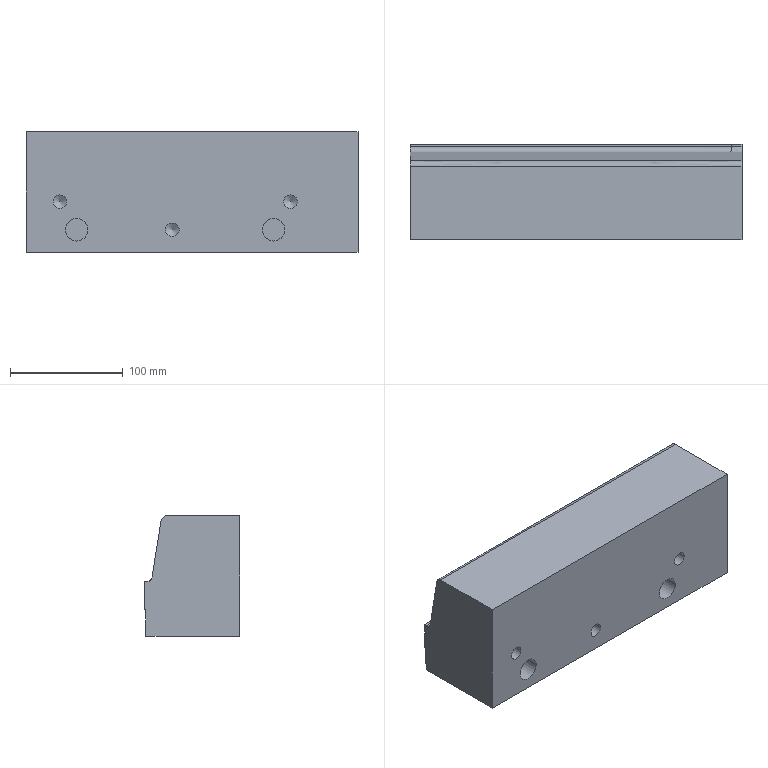Part | NX | features solid 2 | 1 solid | 24 faces | box 295 x 84.705 x 107.133 mm | volume 2449051 mm3 | plane 9 | cylinder 6 | spline 6 | cone 3 | commonest cylinder face diameters 12 x3 20 x2 10 x1
STEP:
#1=CARTESIAN_POINT('',(370.,-160.,-50.));
#2=VERTEX_POINT('',#1);
#3=CARTESIAN_POINT('',(370.,-76.709,-50.));
#4=VERTEX_POINT('',#3);
#5=CARTESIAN_POINT('',(370.,-159.,-50.));
#6=DIRECTION('',(0.,1.,0.));
#7=VECTOR('',#6,1000.);
#8=LINE('',#5,#7);
#9=EDGE_CURVE('',#2,#4,#8,.T.);
#10=ORIENTED_EDGE('',*,*,#9,.T.);
#11=CARTESIAN_POINT('',(665.,-76.708,-50.));
#12=VERTEX_POINT('',#11);
#13=CARTESIAN_POINT('',(370.,-76.709,-50.));
#14=CARTESIAN_POINT('',(468.333,-76.709,-50.));
#15=CARTESIAN_POINT('',(566.667,-76.708,-50.));
#16=CARTESIAN_POINT('',(665.,-76.708,-50.));
#17=B_SPLINE_CURVE_WITH_KNOTS('',3,(#13,#14,#15,#16),.UNSPECIFIED.,.F.,.F.,(4,4),(0.146,0.441),.UNSPECIFIED.);
#18=EDGE_CURVE('',#4,#12,#17,.T.);
#19=ORIENTED_EDGE('',*,*,#18,.T.);
#20=CARTESIAN_POINT('',(665.,-160.,-50.));
#21=VERTEX_POINT('',#20);
#22=CARTESIAN_POINT('',(665.,-74.471,-50.));
#23=DIRECTION('',(0.,1.,0.));
#24=VECTOR('',#23,1000.);
#25=LINE('',#22,#24);
#26=EDGE_CURVE('',#21,#12,#25,.T.);
#27=ORIENTED_EDGE('',*,*,#26,.F.);
#28=CARTESIAN_POINT('',(-571.479,-160.,-50.));
#29=DIRECTION('',(1.,0.,0.));
#30=VECTOR('',#29,1000.);
#31=LINE('',#28,#30);
#32=EDGE_CURVE('',#2,#21,#31,.T.);
#33=ORIENTED_EDGE('',*,*,#32,.F.);
#34=EDGE_LOOP('',(#10,#19,#27,#33));
#35=FACE_BOUND('',#34,.T.);
#36=CARTESIAN_POINT('',(-571.479,-74.471,-50.));
#37=DIRECTION('',(0.,0.,-1.));
#38=DIRECTION('',(-1.,0.,0.));
#39=AXIS2_PLACEMENT_3D('',#36,#37,#38);
#40=PLANE('',#39);
#41=ADVANCED_FACE('',(#35),#40,.T.);
#42=CARTESIAN_POINT('',(415.,-160.,-20.));
#43=VERTEX_POINT('',#42);
#44=CARTESIAN_POINT('',(415.,-160.,-30.));
#45=DIRECTION('',(0.,1.,0.));
#46=DIRECTION('',(0.,0.,1.));
#47=AXIS2_PLACEMENT_3D('',#44,#45,#46);
#48=CIRCLE('',#47,10.);
#49=EDGE_CURVE('',#43,#43,#48,.T.);
#50=ORIENTED_EDGE('',*,*,#49,.T.);
#51=EDGE_LOOP('',(#50));
#52=FACE_BOUND('',#51,.T.);
#53=CARTESIAN_POINT('',(590.,-160.,-20.));
#54=VERTEX_POINT('',#53);
#55=CARTESIAN_POINT('',(590.,-160.,-30.));
#56=DIRECTION('',(0.,1.,0.));
#57=DIRECTION('',(0.,0.,1.));
#58=AXIS2_PLACEMENT_3D('',#55,#56,#57);
#59=CIRCLE('',#58,10.);
#60=EDGE_CURVE('',#54,#54,#59,.T.);
#61=ORIENTED_EDGE('',*,*,#60,.T.);
#62=EDGE_LOOP('',(#61));
#63=FACE_BOUND('',#62,.T.);
#64=CARTESIAN_POINT('',(400.,-160.,1.));
#65=VERTEX_POINT('',#64);
#66=CARTESIAN_POINT('',(400.,-160.,-5.));
#67=DIRECTION('',(0.,1.,0.));
#68=DIRECTION('',(0.,0.,1.));
#69=AXIS2_PLACEMENT_3D('',#66,#67,#68);
#70=CIRCLE('',#69,6.);
#71=EDGE_CURVE('',#65,#65,#70,.T.);
#72=ORIENTED_EDGE('',*,*,#71,.T.);
#73=EDGE_LOOP('',(#72));
#74=FACE_BOUND('',#73,.T.);
#75=CARTESIAN_POINT('',(500.,-160.,-24.));
#76=VERTEX_POINT('',#75);
#77=CARTESIAN_POINT('',(500.,-160.,-30.));
#78=DIRECTION('',(0.,1.,0.));
#79=DIRECTION('',(0.,0.,1.));
#80=AXIS2_PLACEMENT_3D('',#77,#78,#79);
#81=CIRCLE('',#80,6.);
#82=EDGE_CURVE('',#76,#76,#81,.T.);
#83=ORIENTED_EDGE('',*,*,#82,.T.);
#84=EDGE_LOOP('',(#83));
#85=FACE_BOUND('',#84,.T.);
#86=CARTESIAN_POINT('',(605.,-160.,1.));
#87=VERTEX_POINT('',#86);
#88=CARTESIAN_POINT('',(605.,-160.,-5.));
#89=DIRECTION('',(0.,1.,0.));
#90=DIRECTION('',(0.,0.,1.));
#91=AXIS2_PLACEMENT_3D('',#88,#89,#90);
#92=CIRCLE('',#91,6.);
#93=EDGE_CURVE('',#87,#87,#92,.T.);
#94=ORIENTED_EDGE('',*,*,#93,.T.);
#95=EDGE_LOOP('',(#94));
#96=FACE_BOUND('',#95,.T.);
#97=ORIENTED_EDGE('',*,*,#32,.T.);
#98=CARTESIAN_POINT('',(665.,-160.,57.133));
#99=VERTEX_POINT('',#98);
#100=CARTESIAN_POINT('',(665.,-160.,200.));
#101=DIRECTION('',(0.,0.,-1.));
#102=VECTOR('',#101,1000.);
#103=LINE('',#100,#102);
#104=EDGE_CURVE('',#99,#21,#103,.T.);
#105=ORIENTED_EDGE('',*,*,#104,.F.);
#106=CARTESIAN_POINT('',(370.,-160.,57.133));
#107=VERTEX_POINT('',#106);
#108=CARTESIAN_POINT('',(-705.,-160.,57.133));
#109=DIRECTION('',(1.,0.,0.));
#110=VECTOR('',#109,1000.);
#111=LINE('',#108,#110);
#112=EDGE_CURVE('',#107,#99,#111,.T.);
#113=ORIENTED_EDGE('',*,*,#112,.F.);
#114=CARTESIAN_POINT('',(370.,-160.,200.));
#115=DIRECTION('',(0.,0.,1.));
#116=VECTOR('',#115,1000.);
#117=LINE('',#114,#116);
#118=EDGE_CURVE('',#2,#107,#117,.T.);
#119=ORIENTED_EDGE('',*,*,#118,.F.);
#120=EDGE_LOOP('',(#97,#105,#113,#119));
#121=FACE_BOUND('',#120,.T.);
#122=CARTESIAN_POINT('',(-705.,-160.,200.));
#123=DIRECTION('',(0.,1.,0.));
#124=DIRECTION('',(0.,0.,1.));
#125=AXIS2_PLACEMENT_3D('',#122,#123,#124);
#126=PLANE('',#125);
#127=ADVANCED_FACE('',(#52,#63,#74,#85,#96,#121),#126,.F.);
#128=CARTESIAN_POINT('',(370.,-77.294,-1.492));
#129=VERTEX_POINT('',#128);
#130=CARTESIAN_POINT('',(370.,-75.295,-1.509));
#131=VERTEX_POINT('',#130);
#132=CARTESIAN_POINT('',(370.,47.797,-2.56));
#133=DIRECTION('',(0.,1.,-0.008536));
#134=VECTOR('',#133,1000.);
#135=LINE('',#132,#134);
#136=EDGE_CURVE('',#129,#131,#135,.T.);
#137=ORIENTED_EDGE('',*,*,#136,.F.);
#138=CARTESIAN_POINT('',(655.556,-77.294,-1.492));
#139=VERTEX_POINT('',#138);
#140=CARTESIAN_POINT('',(655.556,-77.294,-1.492));
#141=CARTESIAN_POINT('',(560.371,-77.294,-1.492));
#142=CARTESIAN_POINT('',(465.185,-77.294,-1.492));
#143=CARTESIAN_POINT('',(370.,-77.294,-1.492));
#144=B_SPLINE_CURVE_WITH_KNOTS('',3,(#140,#141,#142,#143),.UNSPECIFIED.,.F.,.F.,(4,4),(0.,0.3388),.UNSPECIFIED.);
#145=EDGE_CURVE('',#139,#129,#144,.T.);
#146=ORIENTED_EDGE('',*,*,#145,.F.);
#147=CARTESIAN_POINT('',(655.585,-75.295,-1.509));
#148=VERTEX_POINT('',#147);
#149=CARTESIAN_POINT('',(655.585,-75.295,-1.509));
#150=CARTESIAN_POINT('',(655.576,-75.961,-1.503));
#151=CARTESIAN_POINT('',(655.566,-76.628,-1.498));
#152=CARTESIAN_POINT('',(655.556,-77.294,-1.492));
#153=B_SPLINE_CURVE_WITH_KNOTS('',3,(#149,#150,#151,#152),.UNSPECIFIED.,.F.,.F.,(4,4),(0.8984,1.),.UNSPECIFIED.);
#154=EDGE_CURVE('',#148,#139,#153,.T.);
#155=ORIENTED_EDGE('',*,*,#154,.F.);
#156=CARTESIAN_POINT('',(370.,-75.295,-1.509));
#157=CARTESIAN_POINT('',(465.195,-75.295,-1.509));
#158=CARTESIAN_POINT('',(560.39,-75.295,-1.509));
#159=CARTESIAN_POINT('',(655.585,-75.295,-1.509));
#160=B_SPLINE_CURVE_WITH_KNOTS('',3,(#156,#157,#158,#159),.UNSPECIFIED.,.F.,.F.,(4,4),(0.7675,1.053),.UNSPECIFIED.);
#161=EDGE_CURVE('',#131,#148,#160,.T.);
#162=ORIENTED_EDGE('',*,*,#161,.F.);
#163=EDGE_LOOP('',(#137,#146,#155,#162));
#164=FACE_BOUND('',#163,.T.);
#165=CARTESIAN_POINT('',(35.495,47.797,-2.56));
#166=DIRECTION('',(0.,-0.008536,-1.));
#167=DIRECTION('',(0.,-1.,0.008536));
#168=AXIS2_PLACEMENT_3D('',#165,#166,#167);
#169=PLANE('',#168);
#170=ADVANCED_FACE('',(#164),#169,.F.);
#171=CARTESIAN_POINT('',(370.,-82.189,2.72));
#172=VERTEX_POINT('',#171);
#173=CARTESIAN_POINT('',(370.,-77.252,3.508));
#174=DIRECTION('',(-1.,0.,0.));
#175=DIRECTION('',(0.,0.,1.));
#176=AXIS2_PLACEMENT_3D('',#173,#174,#175);
#177=CIRCLE('',#176,5.);
#178=EDGE_CURVE('',#172,#129,#177,.F.);
#179=ORIENTED_EDGE('',*,*,#178,.F.);
#180=CARTESIAN_POINT('',(655.125,-82.189,2.72));
#181=VERTEX_POINT('',#180);
#182=CARTESIAN_POINT('',(370.,-82.189,2.72));
#183=CARTESIAN_POINT('',(465.042,-82.189,2.72));
#184=CARTESIAN_POINT('',(560.083,-82.189,2.72));
#185=CARTESIAN_POINT('',(655.125,-82.189,2.72));
#186=B_SPLINE_CURVE_WITH_KNOTS('',3,(#182,#183,#184,#185),.UNSPECIFIED.,.F.,.F.,(4,4),(0.6615,1.),.UNSPECIFIED.);
#187=EDGE_CURVE('',#172,#181,#186,.T.);
#188=ORIENTED_EDGE('',*,*,#187,.T.);
#189=CARTESIAN_POINT('',(655.125,-82.189,2.72));
#190=CARTESIAN_POINT('',(655.257,-81.952,1.234));
#191=CARTESIAN_POINT('',(655.46,-80.192,-1.055));
#192=CARTESIAN_POINT('',(655.544,-78.13,-1.485));
#193=CARTESIAN_POINT('',(655.556,-77.294,-1.492));
#194=B_SPLINE_CURVE_WITH_KNOTS('',3,(#189,#190,#191,#192,#193),.UNSPECIFIED.,.F.,.F.,(4,1,4),(0.,0.5,1.),.UNSPECIFIED.);
#195=EDGE_CURVE('',#181,#139,#194,.T.);
#196=ORIENTED_EDGE('',*,*,#195,.T.);
#197=ORIENTED_EDGE('',*,*,#145,.T.);
#198=EDGE_LOOP('',(#179,#188,#196,#197));
#199=FACE_BOUND('',#198,.T.);
#200=CARTESIAN_POINT('',(6000655.556,-77.252,3.508));
#201=DIRECTION('',(-1.,0.,0.));
#202=DIRECTION('',(0.,-0.1575,0.9875));
#203=AXIS2_PLACEMENT_3D('',#200,#201,#202);
#204=CYLINDRICAL_SURFACE('',#203,5.);
#205=ADVANCED_FACE('',(#199),#204,.F.);
#206=CARTESIAN_POINT('',(370.,-90.197,52.92));
#207=VERTEX_POINT('',#206);
#208=CARTESIAN_POINT('',(665.,-90.197,52.92));
#209=VERTEX_POINT('',#208);
#210=CARTESIAN_POINT('',(370.,-90.197,52.92));
#211=CARTESIAN_POINT('',(468.333,-90.197,52.92));
#212=CARTESIAN_POINT('',(566.667,-90.197,52.92));
#213=CARTESIAN_POINT('',(665.,-90.197,52.92));
#214=B_SPLINE_CURVE_WITH_KNOTS('',3,(#210,#211,#212,#213),.UNSPECIFIED.,.F.,.F.,(4,4),(0.5681,0.8631),.UNSPECIFIED.);
#215=EDGE_CURVE('',#207,#209,#214,.T.);
#216=ORIENTED_EDGE('',*,*,#215,.F.);
#217=CARTESIAN_POINT('',(370.,-95.134,57.133));
#218=VERTEX_POINT('',#217);
#219=CARTESIAN_POINT('',(370.,-95.134,52.133));
#220=DIRECTION('',(-1.,0.,0.));
#221=DIRECTION('',(0.,0.,1.));
#222=AXIS2_PLACEMENT_3D('',#219,#220,#221);
#223=CIRCLE('',#222,5.);
#224=EDGE_CURVE('',#207,#218,#223,.F.);
#225=ORIENTED_EDGE('',*,*,#224,.T.);
#226=CARTESIAN_POINT('',(665.,-95.134,57.133));
#227=VERTEX_POINT('',#226);
#228=CARTESIAN_POINT('',(665.,-95.134,57.133));
#229=CARTESIAN_POINT('',(566.667,-95.134,57.133));
#230=CARTESIAN_POINT('',(468.333,-95.134,57.133));
#231=CARTESIAN_POINT('',(370.,-95.134,57.133));
#232=B_SPLINE_CURVE_WITH_KNOTS('',3,(#228,#229,#230,#231),.UNSPECIFIED.,.F.,.F.,(4,4),(0.07861,0.3736),.UNSPECIFIED.);
#233=EDGE_CURVE('',#227,#218,#232,.T.);
#234=ORIENTED_EDGE('',*,*,#233,.F.);
#235=CARTESIAN_POINT('',(665.,-95.134,52.133));
#236=DIRECTION('',(-1.,0.,0.));
#237=DIRECTION('',(0.,0.,1.));
#238=AXIS2_PLACEMENT_3D('',#235,#236,#237);
#239=CIRCLE('',#238,5.);
#240=EDGE_CURVE('',#227,#209,#239,.T.);
#241=ORIENTED_EDGE('',*,*,#240,.T.);
#242=EDGE_LOOP('',(#216,#225,#234,#241));
#243=FACE_BOUND('',#242,.T.);
#244=CARTESIAN_POINT('',(665.,-90.197,52.92));
#245=CARTESIAN_POINT('',(665.,-90.869,57.133));
#246=CARTESIAN_POINT('',(665.,-95.134,57.133));
#247=CARTESIAN_POINT('',(566.667,-90.197,52.92));
#248=CARTESIAN_POINT('',(566.667,-90.869,57.133));
#249=CARTESIAN_POINT('',(566.667,-95.134,57.133));
#250=CARTESIAN_POINT('',(468.333,-90.197,52.92));
#251=CARTESIAN_POINT('',(468.333,-90.869,57.133));
#252=CARTESIAN_POINT('',(468.333,-95.134,57.133));
#253=CARTESIAN_POINT('',(370.,-90.197,52.92));
#254=CARTESIAN_POINT('',(370.,-90.869,57.133));
#255=CARTESIAN_POINT('',(370.,-95.134,57.133));
#256=(BOUNDED_SURFACE()B_SPLINE_SURFACE(3,2,((#244,#245,#246),(#247,#248,#249),(#250,#251,#252),(#253,#254,#255)),.UNSPECIFIED.,.F.,.F.,.F.)B_SPLINE_SURFACE_WITH_KNOTS((4,4),(3,3),(0.1943,0.4893),(0.,1.),.PIECEWISE_BEZIER_KNOTS.)GEOMETRIC_REPRESENTATION_ITEM()RATIONAL_B_SPLINE_SURFACE(((1.,0.7608,1.),(1.,0.7608,1.),(1.,0.7608,1.),(1.,0.7608,1.)))REPRESENTATION_ITEM('')SURFACE());
#257=ADVANCED_FACE('',(#243),#256,.T.);
#258=CARTESIAN_POINT('',(370.,-86.499,29.736));
#259=DIRECTION('',(0.,0.1575,-0.9875));
#260=VECTOR('',#259,1000.);
#261=LINE('',#258,#260);
#262=EDGE_CURVE('',#207,#172,#261,.T.);
#263=ORIENTED_EDGE('',*,*,#262,.F.);
#264=ORIENTED_EDGE('',*,*,#215,.T.);
#265=CARTESIAN_POINT('',(665.,-82.189,2.72));
#266=VERTEX_POINT('',#265);
#267=CARTESIAN_POINT('',(665.,-90.197,52.92));
#268=CARTESIAN_POINT('',(665.,-87.528,36.187));
#269=CARTESIAN_POINT('',(665.,-84.858,19.454));
#270=CARTESIAN_POINT('',(665.,-82.189,2.72));
#271=B_SPLINE_CURVE_WITH_KNOTS('',3,(#267,#268,#269,#270),.UNSPECIFIED.,.F.,.F.,(4,4),(0.1423,0.1932),.UNSPECIFIED.);
#272=EDGE_CURVE('',#266,#209,#271,.F.);
#273=ORIENTED_EDGE('',*,*,#272,.F.);
#274=CARTESIAN_POINT('',(655.125,-82.189,2.72));
#275=CARTESIAN_POINT('',(658.417,-82.189,2.72));
#276=CARTESIAN_POINT('',(661.708,-82.189,2.72));
#277=CARTESIAN_POINT('',(665.,-82.189,2.72));
#278=B_SPLINE_CURVE_WITH_KNOTS('',3,(#274,#275,#276,#277),.UNSPECIFIED.,.F.,.F.,(4,4),(0.9354,0.9453),.UNSPECIFIED.);
#279=EDGE_CURVE('',#181,#266,#278,.T.);
#280=ORIENTED_EDGE('',*,*,#279,.F.);
#281=ORIENTED_EDGE('',*,*,#187,.F.);
#282=EDGE_LOOP('',(#263,#264,#273,#280,#281));
#283=FACE_BOUND('',#282,.T.);
#284=CARTESIAN_POINT('',(808.196,-81.695,-0.3814));
#285=CARTESIAN_POINT('',(-199.284,-81.695,-0.3814));
#286=CARTESIAN_POINT('',(808.196,-91.303,59.853));
#287=CARTESIAN_POINT('',(-199.284,-91.303,59.853));
#288=B_SPLINE_SURFACE_WITH_KNOTS('',1,1,((#284,#285),(#286,#287)),.PLANE_SURF.,.F.,.F.,.F.,(2,2),(2,2),(-0.06964,1.283),(-0.1722,1.),.UNSPECIFIED.);
#289=ADVANCED_FACE('',(#283),#288,.F.);
#290=CARTESIAN_POINT('',(665.,-77.294,-1.492));
#291=VERTEX_POINT('',#290);
#292=CARTESIAN_POINT('',(665.,-77.252,3.508));
#293=DIRECTION('',(-1.,0.,0.));
#294=DIRECTION('',(0.,0.,1.));
#295=AXIS2_PLACEMENT_3D('',#292,#293,#294);
#296=CIRCLE('',#295,5.);
#297=EDGE_CURVE('',#291,#266,#296,.T.);
#298=ORIENTED_EDGE('',*,*,#297,.F.);
#299=CARTESIAN_POINT('',(655.556,-77.294,-1.492));
#300=CARTESIAN_POINT('',(658.704,-77.294,-1.492));
#301=CARTESIAN_POINT('',(661.852,-77.294,-1.492));
#302=CARTESIAN_POINT('',(665.,-77.294,-1.492));
#303=B_SPLINE_CURVE_WITH_KNOTS('',3,(#299,#300,#301,#302),.UNSPECIFIED.,.F.,.F.,(4,4),(0.,0.1078),.UNSPECIFIED.);
#304=EDGE_CURVE('',#139,#291,#303,.T.);
#305=ORIENTED_EDGE('',*,*,#304,.F.);
#306=ORIENTED_EDGE('',*,*,#195,.F.);
#307=ORIENTED_EDGE('',*,*,#279,.T.);
#308=EDGE_LOOP('',(#298,#305,#306,#307));
#309=FACE_BOUND('',#308,.T.);
#310=CARTESIAN_POINT('',(665.,-82.189,2.72));
#311=CARTESIAN_POINT('',(665.,-81.523,-1.456));
#312=CARTESIAN_POINT('',(665.,-77.294,-1.492));
#313=CARTESIAN_POINT('',(661.689,-82.189,2.72));
#314=CARTESIAN_POINT('',(661.689,-81.523,-1.456));
#315=CARTESIAN_POINT('',(661.689,-77.294,-1.492));
#316=CARTESIAN_POINT('',(658.377,-82.189,2.72));
#317=CARTESIAN_POINT('',(658.377,-81.523,-1.456));
#318=CARTESIAN_POINT('',(658.377,-77.294,-1.492));
#319=CARTESIAN_POINT('',(655.066,-82.189,2.72));
#320=CARTESIAN_POINT('',(655.066,-81.523,-1.456));
#321=CARTESIAN_POINT('',(655.066,-77.294,-1.492));
#322=(BOUNDED_SURFACE()B_SPLINE_SURFACE(3,2,((#310,#311,#312),(#313,#314,#315),(#316,#317,#318),(#319,#320,#321)),.UNSPECIFIED.,.F.,.F.,.F.)B_SPLINE_SURFACE_WITH_KNOTS((4,4),(3,3),(0.4081,0.418),(0.,1.),.PIECEWISE_BEZIER_KNOTS.)GEOMETRIC_REPRESENTATION_ITEM()RATIONAL_B_SPLINE_SURFACE(((1.,0.7635,1.),(1.,0.7635,1.),(1.,0.7635,1.),(1.,0.7635,1.)))REPRESENTATION_ITEM('')SURFACE());
#323=ADVANCED_FACE('',(#309),#322,.F.);
#324=CARTESIAN_POINT('',(665.,-75.295,-1.509));
#325=VERTEX_POINT('',#324);
#326=CARTESIAN_POINT('',(655.585,-75.295,-1.509));
#327=CARTESIAN_POINT('',(658.724,-75.295,-1.509));
#328=CARTESIAN_POINT('',(661.862,-75.295,-1.509));
#329=CARTESIAN_POINT('',(665.,-75.295,-1.509));
#330=B_SPLINE_CURVE_WITH_KNOTS('',3,(#326,#327,#328,#329),.UNSPECIFIED.,.F.,.F.,(4,4),(0.000855,0.01027),.UNSPECIFIED.);
#331=EDGE_CURVE('',#148,#325,#330,.T.);
#332=ORIENTED_EDGE('',*,*,#331,.F.);
#333=ORIENTED_EDGE('',*,*,#154,.T.);
#334=ORIENTED_EDGE('',*,*,#304,.T.);
#335=CARTESIAN_POINT('',(665.,-75.295,-1.509));
#336=CARTESIAN_POINT('',(665.,-75.961,-1.503));
#337=CARTESIAN_POINT('',(665.,-76.628,-1.498));
#338=CARTESIAN_POINT('',(665.,-77.294,-1.492));
#339=B_SPLINE_CURVE_WITH_KNOTS('',3,(#335,#336,#337,#338),.UNSPECIFIED.,.F.,.F.,(4,4),(0.01519,0.01719),.UNSPECIFIED.);
#340=EDGE_CURVE('',#325,#291,#339,.T.);
#341=ORIENTED_EDGE('',*,*,#340,.F.);
#342=EDGE_LOOP('',(#332,#333,#334,#341));
#343=FACE_BOUND('',#342,.T.);
#344=CARTESIAN_POINT('',(665.,-75.295,-1.509));
#345=CARTESIAN_POINT('',(655.5,-75.295,-1.509));
#346=CARTESIAN_POINT('',(665.,-77.294,-1.492));
#347=CARTESIAN_POINT('',(655.5,-77.294,-1.492));
#348=B_SPLINE_SURFACE_WITH_KNOTS('',1,1,((#344,#345),(#346,#347)),.PLANE_SURF.,.F.,.F.,.F.,(2,2),(2,2),(0.6913,0.7357),(0.06336,0.0699),.PIECEWISE_BEZIER_KNOTS.);
#349=ADVANCED_FACE('',(#343),#348,.F.);
#350=CARTESIAN_POINT('',(370.,-75.295,-26.51));
#351=VERTEX_POINT('',#350);
#352=CARTESIAN_POINT('',(370.,-75.295,-14.009));
#353=DIRECTION('',(0.,0.,-1.));
#354=VECTOR('',#353,1000.);
#355=LINE('',#352,#354);
#356=EDGE_CURVE('',#131,#351,#355,.T.);
#357=ORIENTED_EDGE('',*,*,#356,.F.);
#358=ORIENTED_EDGE('',*,*,#161,.T.);
#359=ORIENTED_EDGE('',*,*,#331,.T.);
#360=CARTESIAN_POINT('',(665.,-75.295,-26.51));
#361=VERTEX_POINT('',#360);
#362=CARTESIAN_POINT('',(665.,-75.295,-14.009));
#363=DIRECTION('',(0.,0.,-1.));
#364=VECTOR('',#363,1000.);
#365=LINE('',#362,#364);
#366=EDGE_CURVE('',#325,#361,#365,.T.);
#367=ORIENTED_EDGE('',*,*,#366,.T.);
#368=CARTESIAN_POINT('',(665.,-75.295,-26.51));
#369=CARTESIAN_POINT('',(566.667,-75.295,-26.51));
#370=CARTESIAN_POINT('',(468.333,-75.295,-26.51));
#371=CARTESIAN_POINT('',(370.,-75.295,-26.51));
#372=B_SPLINE_CURVE_WITH_KNOTS('',3,(#368,#369,#370,#371),.UNSPECIFIED.,.F.,.F.,(4,4),(-0.005,0.29),.UNSPECIFIED.);
#373=EDGE_CURVE('',#361,#351,#372,.T.);
#374=ORIENTED_EDGE('',*,*,#373,.T.);
#375=EDGE_LOOP('',(#357,#358,#359,#367,#374));
#376=FACE_BOUND('',#375,.T.);
#377=CARTESIAN_POINT('',(665.,-75.295,-1.509));
#378=CARTESIAN_POINT('',(665.,-75.295,-26.51));
#379=CARTESIAN_POINT('',(663.333,-75.295,-1.509));
#380=CARTESIAN_POINT('',(663.333,-75.295,-26.51));
#381=CARTESIAN_POINT('',(661.667,-75.295,-1.509));
#382=CARTESIAN_POINT('',(661.667,-75.295,-26.51));
#383=CARTESIAN_POINT('',(660.,-75.295,-1.509));
#384=CARTESIAN_POINT('',(660.,-75.295,-26.51));
#385=CARTESIAN_POINT('',(563.333,-75.295,-1.509));
#386=CARTESIAN_POINT('',(563.333,-75.295,-26.51));
#387=CARTESIAN_POINT('',(466.667,-75.295,-1.509));
#388=CARTESIAN_POINT('',(466.667,-75.295,-26.51));
#389=CARTESIAN_POINT('',(370.,-75.295,-1.509));
#390=CARTESIAN_POINT('',(370.,-75.295,-26.51));
#391=B_SPLINE_SURFACE_WITH_KNOTS('',3,1,((#377,#378),(#379,#380),(#381,#382),(#383,#384),(#385,#386),(#387,#388),(#389,#390)),.SURF_OF_LINEAR_EXTRUSION.,.F.,.F.,.F.,(4,3,4),(2,2),(-0.003661,0.,0.2124),(0.,1.),.PIECEWISE_BEZIER_KNOTS.);
#392=ADVANCED_FACE('',(#376),#391,.F.);
#393=ORIENTED_EDGE('',*,*,#18,.F.);
#394=CARTESIAN_POINT('',(370.,-76.508,-26.5));
#395=VERTEX_POINT('',#394);
#396=CARTESIAN_POINT('',(370.,-76.709,-50.));
#397=DIRECTION('',(0.,-0.008536,-1.));
#398=VECTOR('',#397,1000.);
#399=LINE('',#396,#398);
#400=EDGE_CURVE('',#4,#395,#399,.F.);
#401=ORIENTED_EDGE('',*,*,#400,.T.);
#402=CARTESIAN_POINT('',(665.,-76.508,-26.5));
#403=VERTEX_POINT('',#402);
#404=CARTESIAN_POINT('',(665.,-76.508,-26.5));
#405=CARTESIAN_POINT('',(566.667,-76.508,-26.5));
#406=CARTESIAN_POINT('',(468.333,-76.508,-26.5));
#407=CARTESIAN_POINT('',(370.,-76.508,-26.5));
#408=B_SPLINE_CURVE_WITH_KNOTS('',3,(#404,#405,#406,#407),.UNSPECIFIED.,.F.,.F.,(4,4),(1.3,1.595),.UNSPECIFIED.);
#409=EDGE_CURVE('',#395,#403,#408,.F.);
#410=ORIENTED_EDGE('',*,*,#409,.T.);
#411=CARTESIAN_POINT('',(665.,-76.608,-38.25));
#412=DIRECTION('',(0.,-0.008536,-1.));
#413=VECTOR('',#412,1000.);
#414=LINE('',#411,#413);
#415=EDGE_CURVE('',#403,#12,#414,.T.);
#416=ORIENTED_EDGE('',*,*,#415,.T.);
#417=EDGE_LOOP('',(#393,#401,#410,#416));
#418=FACE_BOUND('',#417,.T.);
#419=CARTESIAN_POINT('',(370.,-76.508,-26.5));
#420=CARTESIAN_POINT('',(370.,-76.709,-50.));
#421=CARTESIAN_POINT('',(468.333,-76.508,-26.5));
#422=CARTESIAN_POINT('',(468.333,-76.709,-50.));
#423=CARTESIAN_POINT('',(566.667,-76.508,-26.5));
#424=CARTESIAN_POINT('',(566.667,-76.708,-50.));
#425=CARTESIAN_POINT('',(665.,-76.508,-26.5));
#426=CARTESIAN_POINT('',(665.,-76.708,-50.));
#427=B_SPLINE_SURFACE_WITH_KNOTS('',3,1,((#419,#420),(#421,#422),(#423,#424),(#425,#426)),.SURF_OF_LINEAR_EXTRUSION.,.F.,.F.,.F.,(4,4),(2,2),(0.7876,1.004),(0.,1.),.PIECEWISE_BEZIER_KNOTS.);
#428=ADVANCED_FACE('',(#418),#427,.T.);
#429=ORIENTED_EDGE('',*,*,#409,.F.);
#430=CARTESIAN_POINT('',(370.,-75.914,-26.505));
#431=DIRECTION('',(0.,-1.,0.008536));
#432=VECTOR('',#431,1000.);
#433=LINE('',#430,#432);
#434=EDGE_CURVE('',#351,#395,#433,.T.);
#435=ORIENTED_EDGE('',*,*,#434,.F.);
#436=ORIENTED_EDGE('',*,*,#373,.F.);
#437=CARTESIAN_POINT('',(665.,-130.93,-26.035));
#438=DIRECTION('',(0.,1.,-0.008536));
#439=VECTOR('',#438,1000.);
#440=LINE('',#437,#439);
#441=EDGE_CURVE('',#403,#361,#440,.T.);
#442=ORIENTED_EDGE('',*,*,#441,.F.);
#443=EDGE_LOOP('',(#429,#435,#436,#442));
#444=FACE_BOUND('',#443,.T.);
#445=CARTESIAN_POINT('',(-437.652,-75.914,-26.505));
#446=DIRECTION('',(0.,0.008536,1.));
#447=DIRECTION('',(0.,-1.,0.008536));
#448=AXIS2_PLACEMENT_3D('',#445,#446,#447);
#449=PLANE('',#448);
#450=ADVANCED_FACE('',(#444),#449,.F.);
#451=ORIENTED_EDGE('',*,*,#434,.T.);
#452=ORIENTED_EDGE('',*,*,#400,.F.);
#453=ORIENTED_EDGE('',*,*,#9,.F.);
#454=ORIENTED_EDGE('',*,*,#118,.T.);
#455=CARTESIAN_POINT('',(370.,-90.869,57.133));
#456=DIRECTION('',(0.,-1.,0.));
#457=VECTOR('',#456,1000.);
#458=LINE('',#455,#457);
#459=EDGE_CURVE('',#218,#107,#458,.T.);
#460=ORIENTED_EDGE('',*,*,#459,.F.);
#461=ORIENTED_EDGE('',*,*,#224,.F.);
#462=ORIENTED_EDGE('',*,*,#262,.T.);
#463=ORIENTED_EDGE('',*,*,#178,.T.);
#464=ORIENTED_EDGE('',*,*,#136,.T.);
#465=ORIENTED_EDGE('',*,*,#356,.T.);
#466=EDGE_LOOP('',(#451,#452,#453,#454,#460,#461,#462,#463,#464,#465));
#467=FACE_BOUND('',#466,.T.);
#468=CARTESIAN_POINT('',(370.,361.,0.));
#469=DIRECTION('',(-1.,0.,0.));
#470=DIRECTION('',(0.,0.,1.));
#471=AXIS2_PLACEMENT_3D('',#468,#469,#470);
#472=PLANE('',#471);
#473=ADVANCED_FACE('',(#467),#472,.T.);
#474=ORIENTED_EDGE('',*,*,#233,.T.);
#475=ORIENTED_EDGE('',*,*,#459,.T.);
#476=ORIENTED_EDGE('',*,*,#112,.T.);
#477=CARTESIAN_POINT('',(665.,-129.,57.133));
#478=DIRECTION('',(0.,1.,0.));
#479=VECTOR('',#478,1000.);
#480=LINE('',#477,#479);
#481=EDGE_CURVE('',#99,#227,#480,.T.);
#482=ORIENTED_EDGE('',*,*,#481,.T.);
#483=EDGE_LOOP('',(#474,#475,#476,#482));
#484=FACE_BOUND('',#483,.T.);
#485=CARTESIAN_POINT('',(743.607,-90.869,57.133));
#486=DIRECTION('',(0.,0.,1.));
#487=DIRECTION('',(1.,0.,0.));
#488=AXIS2_PLACEMENT_3D('',#485,#486,#487);
#489=PLANE('',#488);
#490=ADVANCED_FACE('',(#484),#489,.T.);
#491=ORIENTED_EDGE('',*,*,#104,.T.);
#492=ORIENTED_EDGE('',*,*,#26,.T.);
#493=ORIENTED_EDGE('',*,*,#415,.F.);
#494=ORIENTED_EDGE('',*,*,#441,.T.);
#495=ORIENTED_EDGE('',*,*,#366,.F.);
#496=ORIENTED_EDGE('',*,*,#340,.T.);
#497=ORIENTED_EDGE('',*,*,#297,.T.);
#498=ORIENTED_EDGE('',*,*,#272,.T.);
#499=ORIENTED_EDGE('',*,*,#240,.F.);
#500=ORIENTED_EDGE('',*,*,#481,.F.);
#501=EDGE_LOOP('',(#491,#492,#493,#494,#495,#496,#497,#498,#499,#500));
#502=FACE_BOUND('',#501,.T.);
#503=CARTESIAN_POINT('',(665.,-129.,200.));
#504=DIRECTION('',(-1.,0.,0.));
#505=DIRECTION('',(0.,0.,1.));
#506=AXIS2_PLACEMENT_3D('',#503,#504,#505);
#507=PLANE('',#506);
#508=ADVANCED_FACE('',(#502),#507,.F.);
#509=CARTESIAN_POINT('',(605.,-129.,1.));
#510=VERTEX_POINT('',#509);
#511=CARTESIAN_POINT('',(605.,-129.,-5.));
#512=DIRECTION('',(0.,1.,0.));
#513=DIRECTION('',(0.,0.,1.));
#514=AXIS2_PLACEMENT_3D('',#511,#512,#513);
#515=CIRCLE('',#514,6.);
#516=EDGE_CURVE('',#510,#510,#515,.T.);
#517=ORIENTED_EDGE('',*,*,#516,.F.);
#518=EDGE_LOOP('',(#517));
#519=FACE_BOUND('',#518,.T.);
#520=CARTESIAN_POINT('',(605.,-125.395,-5.));
#521=VERTEX_POINT('',#520);
#522=VERTEX_LOOP('',#521);
#523=FACE_BOUND('',#522,.T.);
#524=CARTESIAN_POINT('',(605.,-129.,-5.));
#525=DIRECTION('',(0.,-1.,0.));
#526=DIRECTION('',(0.,0.,-1.));
#527=AXIS2_PLACEMENT_3D('',#524,#525,#526);
#528=CONICAL_SURFACE('',#527,6.,1.03);
#529=ADVANCED_FACE('',(#519,#523),#528,.F.);
#530=ORIENTED_EDGE('',*,*,#516,.T.);
#531=EDGE_LOOP('',(#530));
#532=FACE_BOUND('',#531,.T.);
#533=ORIENTED_EDGE('',*,*,#93,.F.);
#534=EDGE_LOOP('',(#533));
#535=FACE_BOUND('',#534,.T.);
#536=CARTESIAN_POINT('',(605.,-159.,-5.));
#537=DIRECTION('',(0.,1.,0.));
#538=DIRECTION('',(0.,0.,1.));
#539=AXIS2_PLACEMENT_3D('',#536,#537,#538);
#540=CYLINDRICAL_SURFACE('',#539,6.);
#541=ADVANCED_FACE('',(#532,#535),#540,.F.);
#542=CARTESIAN_POINT('',(500.,-129.,-24.));
#543=VERTEX_POINT('',#542);
#544=CARTESIAN_POINT('',(500.,-129.,-30.));
#545=DIRECTION('',(0.,1.,0.));
#546=DIRECTION('',(0.,0.,1.));
#547=AXIS2_PLACEMENT_3D('',#544,#545,#546);
#548=CIRCLE('',#547,6.);
#549=EDGE_CURVE('',#543,#543,#548,.T.);
#550=ORIENTED_EDGE('',*,*,#549,.F.);
#551=EDGE_LOOP('',(#550));
#552=FACE_BOUND('',#551,.T.);
#553=CARTESIAN_POINT('',(500.,-125.395,-30.));
#554=VERTEX_POINT('',#553);
#555=VERTEX_LOOP('',#554);
#556=FACE_BOUND('',#555,.T.);
#557=CARTESIAN_POINT('',(500.,-129.,-30.));
#558=DIRECTION('',(0.,-1.,0.));
#559=DIRECTION('',(0.,0.,-1.));
#560=AXIS2_PLACEMENT_3D('',#557,#558,#559);
#561=CONICAL_SURFACE('',#560,6.,1.03);
#562=ADVANCED_FACE('',(#552,#556),#561,.F.);
#563=ORIENTED_EDGE('',*,*,#549,.T.);
#564=EDGE_LOOP('',(#563));
#565=FACE_BOUND('',#564,.T.);
#566=ORIENTED_EDGE('',*,*,#82,.F.);
#567=EDGE_LOOP('',(#566));
#568=FACE_BOUND('',#567,.T.);
#569=CARTESIAN_POINT('',(500.,-159.,-30.));
#570=DIRECTION('',(0.,1.,0.));
#571=DIRECTION('',(0.,0.,1.));
#572=AXIS2_PLACEMENT_3D('',#569,#570,#571);
#573=CYLINDRICAL_SURFACE('',#572,6.);
#574=ADVANCED_FACE('',(#565,#568),#573,.F.);
#575=CARTESIAN_POINT('',(400.,-129.,1.));
#576=VERTEX_POINT('',#575);
#577=CARTESIAN_POINT('',(400.,-129.,-5.));
#578=DIRECTION('',(0.,1.,0.));
#579=DIRECTION('',(0.,0.,1.));
#580=AXIS2_PLACEMENT_3D('',#577,#578,#579);
#581=CIRCLE('',#580,6.);
#582=EDGE_CURVE('',#576,#576,#581,.T.);
#583=ORIENTED_EDGE('',*,*,#582,.F.);
#584=EDGE_LOOP('',(#583));
#585=FACE_BOUND('',#584,.T.);
#586=CARTESIAN_POINT('',(400.,-125.395,-5.));
#587=VERTEX_POINT('',#586);
#588=VERTEX_LOOP('',#587);
#589=FACE_BOUND('',#588,.T.);
#590=CARTESIAN_POINT('',(400.,-129.,-5.));
#591=DIRECTION('',(0.,-1.,0.));
#592=DIRECTION('',(0.,0.,-1.));
#593=AXIS2_PLACEMENT_3D('',#590,#591,#592);
#594=CONICAL_SURFACE('',#593,6.,1.03);
#595=ADVANCED_FACE('',(#585,#589),#594,.F.);
#596=ORIENTED_EDGE('',*,*,#582,.T.);
#597=EDGE_LOOP('',(#596));
#598=FACE_BOUND('',#597,.T.);
#599=ORIENTED_EDGE('',*,*,#71,.F.);
#600=EDGE_LOOP('',(#599));
#601=FACE_BOUND('',#600,.T.);
#602=CARTESIAN_POINT('',(400.,-159.,-5.));
#603=DIRECTION('',(0.,1.,0.));
#604=DIRECTION('',(0.,0.,1.));
#605=AXIS2_PLACEMENT_3D('',#602,#603,#604);
#606=CYLINDRICAL_SURFACE('',#605,6.);
#607=ADVANCED_FACE('',(#598,#601),#606,.F.);
#608=CARTESIAN_POINT('',(590.,-129.,-20.));
#609=VERTEX_POINT('',#608);
#610=CARTESIAN_POINT('',(590.,-129.,-30.));
#611=DIRECTION('',(0.,1.,0.));
#612=DIRECTION('',(0.,0.,1.));
#613=AXIS2_PLACEMENT_3D('',#610,#611,#612);
#614=CIRCLE('',#613,10.);
#615=EDGE_CURVE('',#609,#609,#614,.T.);
#616=ORIENTED_EDGE('',*,*,#615,.T.);
#617=EDGE_LOOP('',(#616));
#618=FACE_BOUND('',#617,.T.);
#619=ORIENTED_EDGE('',*,*,#60,.F.);
#620=EDGE_LOOP('',(#619));
#621=FACE_BOUND('',#620,.T.);
#622=CARTESIAN_POINT('',(590.,-159.,-30.));
#623=DIRECTION('',(0.,1.,0.));
#624=DIRECTION('',(0.,0.,1.));
#625=AXIS2_PLACEMENT_3D('',#622,#623,#624);
#626=CYLINDRICAL_SURFACE('',#625,10.);
#627=ADVANCED_FACE('',(#618,#621),#626,.F.);
#628=ORIENTED_EDGE('',*,*,#615,.F.);
#629=EDGE_LOOP('',(#628));
#630=FACE_BOUND('',#629,.T.);
#631=CARTESIAN_POINT('',(590.,-129.,-30.));
#632=DIRECTION('',(0.,1.,0.));
#633=DIRECTION('',(0.,0.,1.));
#634=AXIS2_PLACEMENT_3D('',#631,#632,#633);
#635=PLANE('',#634);
#636=ADVANCED_FACE('',(#630),#635,.F.);
#637=CARTESIAN_POINT('',(415.,-129.,-20.));
#638=VERTEX_POINT('',#637);
#639=CARTESIAN_POINT('',(415.,-129.,-30.));
#640=DIRECTION('',(0.,1.,0.));
#641=DIRECTION('',(0.,0.,1.));
#642=AXIS2_PLACEMENT_3D('',#639,#640,#641);
#643=CIRCLE('',#642,10.);
#644=EDGE_CURVE('',#638,#638,#643,.T.);
#645=ORIENTED_EDGE('',*,*,#644,.T.);
#646=EDGE_LOOP('',(#645));
#647=FACE_BOUND('',#646,.T.);
#648=ORIENTED_EDGE('',*,*,#49,.F.);
#649=EDGE_LOOP('',(#648));
#650=FACE_BOUND('',#649,.T.);
#651=CARTESIAN_POINT('',(415.,-159.,-30.));
#652=DIRECTION('',(0.,1.,0.));
#653=DIRECTION('',(0.,0.,1.));
#654=AXIS2_PLACEMENT_3D('',#651,#652,#653);
#655=CYLINDRICAL_SURFACE('',#654,10.);
#656=ADVANCED_FACE('',(#647,#650),#655,.F.);
#657=ORIENTED_EDGE('',*,*,#644,.F.);
#658=EDGE_LOOP('',(#657));
#659=FACE_BOUND('',#658,.T.);
#660=CARTESIAN_POINT('',(415.,-129.,-30.));
#661=DIRECTION('',(0.,1.,0.));
#662=DIRECTION('',(0.,0.,1.));
#663=AXIS2_PLACEMENT_3D('',#660,#661,#662);
#664=PLANE('',#663);
#665=ADVANCED_FACE('',(#659),#664,.F.);
#666=CLOSED_SHELL('',(#41,#127,#170,#205,#257,#289,#323,#349,#392,#428,#450,#473,#490,#508,#529,#541,#562,#574,#595,#607,#627,#636,#656,#665));
#667=MANIFOLD_SOLID_BREP('',#666);
#668=(LENGTH_UNIT()NAMED_UNIT(*)SI_UNIT(.MILLI.,.METRE.));
#669=UNCERTAINTY_MEASURE_WITH_UNIT(LENGTH_MEASURE(0.0508),#668,'','');
#670=(NAMED_UNIT(*)PLANE_ANGLE_UNIT()SI_UNIT($,.RADIAN.));
#671=(NAMED_UNIT(*)SI_UNIT($,.STERADIAN.)SOLID_ANGLE_UNIT());
#672=(GEOMETRIC_REPRESENTATION_CONTEXT(3)GLOBAL_UNCERTAINTY_ASSIGNED_CONTEXT((#669))GLOBAL_UNIT_ASSIGNED_CONTEXT((#668,#670,#671))REPRESENTATION_CONTEXT('',''));
#673=ADVANCED_BREP_SHAPE_REPRESENTATION('',(#667),#672);